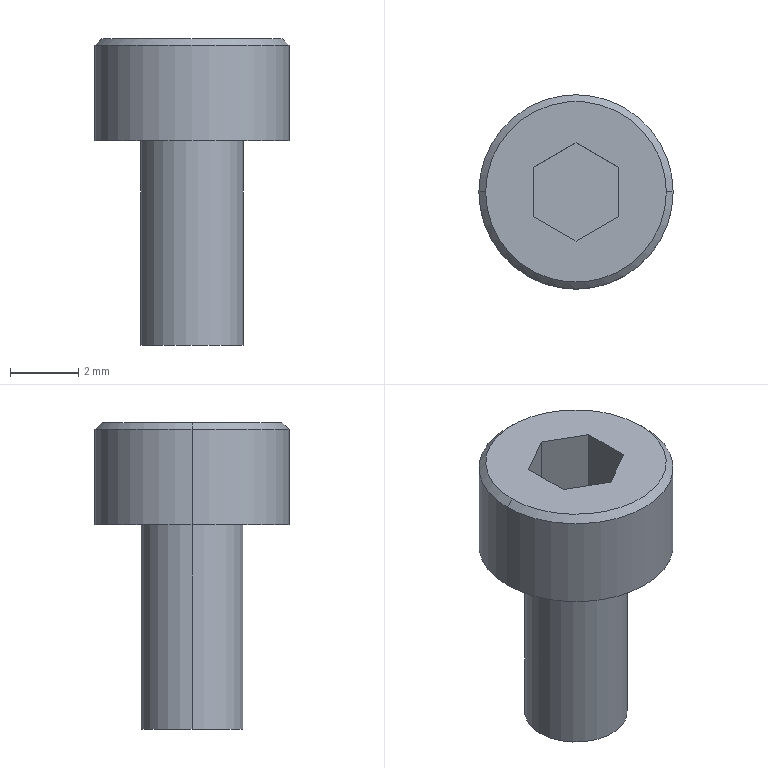Part | SolidWorks | features ICE 2, Chamfer 1, Extrusion 1 | 1 solid | 16 faces | box 5.7 x 5.7 x 9 mm | volume 102.377 mm3 | plane 10 | cylinder 4 | cone 2 | commonest cylinder face diameters 3 x2 5.7 x2
STEP:
#1=CARTESIAN_POINT('',(-1.5,0.,-6.));
#2=VERTEX_POINT('',#1);
#3=CARTESIAN_POINT('',(1.5,0.,-6.));
#4=VERTEX_POINT('',#3);
#5=CARTESIAN_POINT('',(0.,0.,-6.));
#6=DIRECTION('',(0.,0.,-1.));
#7=DIRECTION('',(-1.,0.,0.));
#8=AXIS2_PLACEMENT_3D('',#5,#6,#7);
#9=CIRCLE('',#8,1.5);
#10=EDGE_CURVE('',#2,#4,#9,.T.);
#11=ORIENTED_EDGE('',*,*,#10,.F.);
#12=CARTESIAN_POINT('',(-1.5,0.,0.));
#13=VERTEX_POINT('',#12);
#14=CARTESIAN_POINT('',(-1.5,0.,-6.));
#15=DIRECTION('',(0.,0.,1.));
#16=VECTOR('',#15,1000.);
#17=LINE('',#14,#16);
#18=EDGE_CURVE('',#2,#13,#17,.T.);
#19=ORIENTED_EDGE('',*,*,#18,.T.);
#20=CARTESIAN_POINT('',(1.5,0.,0.));
#21=VERTEX_POINT('',#20);
#22=CARTESIAN_POINT('',(0.,0.,0.));
#23=DIRECTION('',(0.,0.,-1.));
#24=DIRECTION('',(1.,0.,0.));
#25=AXIS2_PLACEMENT_3D('',#22,#23,#24);
#26=CIRCLE('',#25,1.5);
#27=EDGE_CURVE('',#13,#21,#26,.T.);
#28=ORIENTED_EDGE('',*,*,#27,.T.);
#29=CARTESIAN_POINT('',(1.5,0.,-6.));
#30=DIRECTION('',(0.,0.,1.));
#31=VECTOR('',#30,1000.);
#32=LINE('',#29,#31);
#33=EDGE_CURVE('',#4,#21,#32,.T.);
#34=ORIENTED_EDGE('',*,*,#33,.F.);
#35=EDGE_LOOP('',(#11,#19,#28,#34));
#36=FACE_OUTER_BOUND('',#35,.T.);
#37=CARTESIAN_POINT('',(0.,0.,-6.));
#38=DIRECTION('',(0.,0.,1.));
#39=DIRECTION('',(1.,0.,0.));
#40=AXIS2_PLACEMENT_3D('',#37,#38,#39);
#41=CYLINDRICAL_SURFACE('',#40,1.5);
#42=ADVANCED_FACE('',(#36),#41,.T.);
#43=CARTESIAN_POINT('',(2.65,0.,3.));
#44=VERTEX_POINT('',#43);
#45=CARTESIAN_POINT('',(-2.65,0.,3.));
#46=VERTEX_POINT('',#45);
#47=CARTESIAN_POINT('',(0.,0.,3.));
#48=DIRECTION('',(0.,0.,1.));
#49=DIRECTION('',(1.,0.,0.));
#50=AXIS2_PLACEMENT_3D('',#47,#48,#49);
#51=CIRCLE('',#50,2.65);
#52=EDGE_CURVE('',#44,#46,#51,.T.);
#53=ORIENTED_EDGE('',*,*,#52,.F.);
#54=CARTESIAN_POINT('',(2.85,0.,2.8));
#55=VERTEX_POINT('',#54);
#56=CARTESIAN_POINT('',(2.65,0.,3.));
#57=DIRECTION('',(0.7071,0.,-0.7071));
#58=VECTOR('',#57,1000.);
#59=LINE('',#56,#58);
#60=EDGE_CURVE('',#44,#55,#59,.T.);
#61=ORIENTED_EDGE('',*,*,#60,.T.);
#62=CARTESIAN_POINT('',(-2.85,0.,2.8));
#63=VERTEX_POINT('',#62);
#64=CARTESIAN_POINT('',(0.,0.,2.8));
#65=DIRECTION('',(0.,0.,-1.));
#66=DIRECTION('',(1.,0.,0.));
#67=AXIS2_PLACEMENT_3D('',#64,#65,#66);
#68=CIRCLE('',#67,2.85);
#69=EDGE_CURVE('',#63,#55,#68,.T.);
#70=ORIENTED_EDGE('',*,*,#69,.F.);
#71=CARTESIAN_POINT('',(-2.65,0.,3.));
#72=DIRECTION('',(-0.7071,0.,-0.7071));
#73=VECTOR('',#72,1000.);
#74=LINE('',#71,#73);
#75=EDGE_CURVE('',#46,#63,#74,.T.);
#76=ORIENTED_EDGE('',*,*,#75,.F.);
#77=EDGE_LOOP('',(#53,#61,#70,#76));
#78=FACE_OUTER_BOUND('',#77,.T.);
#79=CARTESIAN_POINT('',(0.,0.,3.));
#80=DIRECTION('',(0.,0.,-1.));
#81=DIRECTION('',(-1.,0.,0.));
#82=AXIS2_PLACEMENT_3D('',#79,#80,#81);
#83=CONICAL_SURFACE('',#82,2.65,0.7854);
#84=ADVANCED_FACE('',(#78),#83,.T.);
#85=ORIENTED_EDGE('',*,*,#69,.T.);
#86=CARTESIAN_POINT('',(2.85,0.,0.));
#87=VERTEX_POINT('',#86);
#88=CARTESIAN_POINT('',(2.85,0.,3.));
#89=DIRECTION('',(0.,0.,-1.));
#90=VECTOR('',#89,1000.);
#91=LINE('',#88,#90);
#92=EDGE_CURVE('',#55,#87,#91,.T.);
#93=ORIENTED_EDGE('',*,*,#92,.T.);
#94=CARTESIAN_POINT('',(-2.85,0.,0.));
#95=VERTEX_POINT('',#94);
#96=CARTESIAN_POINT('',(0.,0.,0.));
#97=DIRECTION('',(0.,0.,1.));
#98=DIRECTION('',(1.,0.,0.));
#99=AXIS2_PLACEMENT_3D('',#96,#97,#98);
#100=CIRCLE('',#99,2.85);
#101=EDGE_CURVE('',#87,#95,#100,.T.);
#102=ORIENTED_EDGE('',*,*,#101,.T.);
#103=CARTESIAN_POINT('',(-2.85,0.,3.));
#104=DIRECTION('',(0.,0.,-1.));
#105=VECTOR('',#104,1000.);
#106=LINE('',#103,#105);
#107=EDGE_CURVE('',#63,#95,#106,.T.);
#108=ORIENTED_EDGE('',*,*,#107,.F.);
#109=EDGE_LOOP('',(#85,#93,#102,#108));
#110=FACE_OUTER_BOUND('',#109,.T.);
#111=CARTESIAN_POINT('',(0.,0.,3.));
#112=DIRECTION('',(0.,0.,-1.));
#113=DIRECTION('',(-1.,0.,0.));
#114=AXIS2_PLACEMENT_3D('',#111,#112,#113);
#115=CYLINDRICAL_SURFACE('',#114,2.85);
#116=ADVANCED_FACE('',(#110),#115,.T.);
#117=CARTESIAN_POINT('',(0.,0.,0.));
#118=DIRECTION('',(0.,0.,1.));
#119=DIRECTION('',(1.,0.,0.));
#120=AXIS2_PLACEMENT_3D('',#117,#118,#119);
#121=CIRCLE('',#120,2.85);
#122=EDGE_CURVE('',#95,#87,#121,.T.);
#123=ORIENTED_EDGE('',*,*,#122,.F.);
#124=ORIENTED_EDGE('',*,*,#101,.F.);
#125=EDGE_LOOP('',(#123,#124));
#126=FACE_OUTER_BOUND('',#125,.T.);
#127=CARTESIAN_POINT('',(0.,0.,0.));
#128=DIRECTION('',(0.,0.,-1.));
#129=DIRECTION('',(1.,0.,0.));
#130=AXIS2_PLACEMENT_3D('',#127,#128,#129);
#131=CIRCLE('',#130,1.5);
#132=EDGE_CURVE('',#21,#13,#131,.T.);
#133=ORIENTED_EDGE('',*,*,#132,.F.);
#134=ORIENTED_EDGE('',*,*,#27,.F.);
#135=EDGE_LOOP('',(#133,#134));
#136=FACE_BOUND('',#135,.T.);
#137=CARTESIAN_POINT('',(0.,0.,0.));
#138=DIRECTION('',(0.,0.,1.));
#139=DIRECTION('',(1.,0.,0.));
#140=AXIS2_PLACEMENT_3D('',#137,#138,#139);
#141=PLANE('',#140);
#142=ADVANCED_FACE('',(#126,#136),#141,.F.);
#143=ORIENTED_EDGE('',*,*,#92,.F.);
#144=CARTESIAN_POINT('',(0.,0.,2.8));
#145=DIRECTION('',(0.,0.,-1.));
#146=DIRECTION('',(1.,0.,0.));
#147=AXIS2_PLACEMENT_3D('',#144,#145,#146);
#148=CIRCLE('',#147,2.85);
#149=EDGE_CURVE('',#55,#63,#148,.T.);
#150=ORIENTED_EDGE('',*,*,#149,.T.);
#151=ORIENTED_EDGE('',*,*,#107,.T.);
#152=ORIENTED_EDGE('',*,*,#122,.T.);
#153=EDGE_LOOP('',(#143,#150,#151,#152));
#154=FACE_OUTER_BOUND('',#153,.T.);
#155=CARTESIAN_POINT('',(0.,0.,3.));
#156=DIRECTION('',(0.,0.,-1.));
#157=DIRECTION('',(-1.,0.,0.));
#158=AXIS2_PLACEMENT_3D('',#155,#156,#157);
#159=CYLINDRICAL_SURFACE('',#158,2.85);
#160=ADVANCED_FACE('',(#154),#159,.T.);
#161=CARTESIAN_POINT('',(0.,0.,3.));
#162=DIRECTION('',(0.,0.,1.));
#163=DIRECTION('',(1.,0.,0.));
#164=AXIS2_PLACEMENT_3D('',#161,#162,#163);
#165=CIRCLE('',#164,2.65);
#166=EDGE_CURVE('',#46,#44,#165,.T.);
#167=ORIENTED_EDGE('',*,*,#166,.T.);
#168=ORIENTED_EDGE('',*,*,#52,.T.);
#169=EDGE_LOOP('',(#167,#168));
#170=FACE_OUTER_BOUND('',#169,.T.);
#171=CARTESIAN_POINT('',(1.25,0.7217,3.));
#172=VERTEX_POINT('',#171);
#173=CARTESIAN_POINT('',(0.,1.443,3.));
#174=VERTEX_POINT('',#173);
#175=CARTESIAN_POINT('',(1.25,0.7217,3.));
#176=DIRECTION('',(-0.866,0.5,0.));
#177=VECTOR('',#176,1000.);
#178=LINE('',#175,#177);
#179=EDGE_CURVE('',#172,#174,#178,.T.);
#180=ORIENTED_EDGE('',*,*,#179,.F.);
#181=CARTESIAN_POINT('',(1.25,-0.7217,3.));
#182=VERTEX_POINT('',#181);
#183=CARTESIAN_POINT('',(1.25,-0.7217,3.));
#184=DIRECTION('',(0.,1.,0.));
#185=VECTOR('',#184,1000.);
#186=LINE('',#183,#185);
#187=EDGE_CURVE('',#182,#172,#186,.T.);
#188=ORIENTED_EDGE('',*,*,#187,.F.);
#189=CARTESIAN_POINT('',(0.,-1.443,3.));
#190=VERTEX_POINT('',#189);
#191=CARTESIAN_POINT('',(0.,-1.443,3.));
#192=DIRECTION('',(0.866,0.5,0.));
#193=VECTOR('',#192,1000.);
#194=LINE('',#191,#193);
#195=EDGE_CURVE('',#190,#182,#194,.T.);
#196=ORIENTED_EDGE('',*,*,#195,.F.);
#197=CARTESIAN_POINT('',(-1.25,-0.7217,3.));
#198=VERTEX_POINT('',#197);
#199=CARTESIAN_POINT('',(-1.25,-0.7217,3.));
#200=DIRECTION('',(0.866,-0.5,0.));
#201=VECTOR('',#200,1000.);
#202=LINE('',#199,#201);
#203=EDGE_CURVE('',#198,#190,#202,.T.);
#204=ORIENTED_EDGE('',*,*,#203,.F.);
#205=CARTESIAN_POINT('',(-1.25,0.7217,3.));
#206=VERTEX_POINT('',#205);
#207=CARTESIAN_POINT('',(-1.25,0.7217,3.));
#208=DIRECTION('',(0.,-1.,0.));
#209=VECTOR('',#208,1000.);
#210=LINE('',#207,#209);
#211=EDGE_CURVE('',#206,#198,#210,.T.);
#212=ORIENTED_EDGE('',*,*,#211,.F.);
#213=CARTESIAN_POINT('',(0.,1.443,3.));
#214=DIRECTION('',(-0.866,-0.5,0.));
#215=VECTOR('',#214,1000.);
#216=LINE('',#213,#215);
#217=EDGE_CURVE('',#174,#206,#216,.T.);
#218=ORIENTED_EDGE('',*,*,#217,.F.);
#219=EDGE_LOOP('',(#180,#188,#196,#204,#212,#218));
#220=FACE_BOUND('',#219,.T.);
#221=CARTESIAN_POINT('',(0.,0.,3.));
#222=DIRECTION('',(0.,0.,1.));
#223=DIRECTION('',(1.,0.,0.));
#224=AXIS2_PLACEMENT_3D('',#221,#222,#223);
#225=PLANE('',#224);
#226=ADVANCED_FACE('',(#170,#220),#225,.T.);
#227=CARTESIAN_POINT('',(1.25,0.7217,0.));
#228=VERTEX_POINT('',#227);
#229=CARTESIAN_POINT('',(1.25,0.7217,-1.));
#230=DIRECTION('',(0.,0.,1.));
#231=VECTOR('',#230,1000.);
#232=LINE('',#229,#231);
#233=EDGE_CURVE('',#228,#172,#232,.T.);
#234=ORIENTED_EDGE('',*,*,#233,.T.);
#235=ORIENTED_EDGE('',*,*,#179,.T.);
#236=CARTESIAN_POINT('',(0.,1.443,0.));
#237=VERTEX_POINT('',#236);
#238=CARTESIAN_POINT('',(0.,1.443,-1.));
#239=DIRECTION('',(0.,0.,1.));
#240=VECTOR('',#239,1000.);
#241=LINE('',#238,#240);
#242=EDGE_CURVE('',#237,#174,#241,.T.);
#243=ORIENTED_EDGE('',*,*,#242,.F.);
#244=CARTESIAN_POINT('',(0.625,1.083,0.));
#245=DIRECTION('',(-0.866,0.5,0.));
#246=VECTOR('',#245,1000.);
#247=LINE('',#244,#246);
#248=EDGE_CURVE('',#228,#237,#247,.T.);
#249=ORIENTED_EDGE('',*,*,#248,.F.);
#250=EDGE_LOOP('',(#234,#235,#243,#249));
#251=FACE_OUTER_BOUND('',#250,.T.);
#252=CARTESIAN_POINT('',(1.25,0.7217,-1.));
#253=DIRECTION('',(0.5,0.866,0.));
#254=DIRECTION('',(-0.866,0.5,0.));
#255=AXIS2_PLACEMENT_3D('',#252,#253,#254);
#256=PLANE('',#255);
#257=ADVANCED_FACE('',(#251),#256,.F.);
#258=CARTESIAN_POINT('',(1.25,-0.7217,0.));
#259=VERTEX_POINT('',#258);
#260=CARTESIAN_POINT('',(1.25,-0.7217,-1.));
#261=DIRECTION('',(0.,0.,1.));
#262=VECTOR('',#261,1000.);
#263=LINE('',#260,#262);
#264=EDGE_CURVE('',#259,#182,#263,.T.);
#265=ORIENTED_EDGE('',*,*,#264,.T.);
#266=ORIENTED_EDGE('',*,*,#187,.T.);
#267=ORIENTED_EDGE('',*,*,#233,.F.);
#268=CARTESIAN_POINT('',(1.25,0.,0.));
#269=DIRECTION('',(0.,1.,0.));
#270=VECTOR('',#269,1000.);
#271=LINE('',#268,#270);
#272=EDGE_CURVE('',#259,#228,#271,.T.);
#273=ORIENTED_EDGE('',*,*,#272,.F.);
#274=EDGE_LOOP('',(#265,#266,#267,#273));
#275=FACE_OUTER_BOUND('',#274,.T.);
#276=CARTESIAN_POINT('',(1.25,-0.7217,-1.));
#277=DIRECTION('',(1.,0.,0.));
#278=DIRECTION('',(0.,1.,0.));
#279=AXIS2_PLACEMENT_3D('',#276,#277,#278);
#280=PLANE('',#279);
#281=ADVANCED_FACE('',(#275),#280,.F.);
#282=CARTESIAN_POINT('',(0.,-1.443,0.));
#283=VERTEX_POINT('',#282);
#284=CARTESIAN_POINT('',(0.,-1.443,-1.));
#285=DIRECTION('',(0.,0.,1.));
#286=VECTOR('',#285,1000.);
#287=LINE('',#284,#286);
#288=EDGE_CURVE('',#283,#190,#287,.T.);
#289=ORIENTED_EDGE('',*,*,#288,.T.);
#290=ORIENTED_EDGE('',*,*,#195,.T.);
#291=ORIENTED_EDGE('',*,*,#264,.F.);
#292=CARTESIAN_POINT('',(0.625,-1.083,0.));
#293=DIRECTION('',(0.866,0.5,0.));
#294=VECTOR('',#293,1000.);
#295=LINE('',#292,#294);
#296=EDGE_CURVE('',#283,#259,#295,.T.);
#297=ORIENTED_EDGE('',*,*,#296,.F.);
#298=EDGE_LOOP('',(#289,#290,#291,#297));
#299=FACE_OUTER_BOUND('',#298,.T.);
#300=CARTESIAN_POINT('',(0.,-1.443,-1.));
#301=DIRECTION('',(0.5,-0.866,0.));
#302=DIRECTION('',(0.866,0.5,0.));
#303=AXIS2_PLACEMENT_3D('',#300,#301,#302);
#304=PLANE('',#303);
#305=ADVANCED_FACE('',(#299),#304,.F.);
#306=CARTESIAN_POINT('',(-1.25,-0.7217,0.));
#307=VERTEX_POINT('',#306);
#308=CARTESIAN_POINT('',(-1.25,-0.7217,-1.));
#309=DIRECTION('',(0.,0.,1.));
#310=VECTOR('',#309,1000.);
#311=LINE('',#308,#310);
#312=EDGE_CURVE('',#307,#198,#311,.T.);
#313=ORIENTED_EDGE('',*,*,#312,.T.);
#314=ORIENTED_EDGE('',*,*,#203,.T.);
#315=ORIENTED_EDGE('',*,*,#288,.F.);
#316=CARTESIAN_POINT('',(-0.625,-1.083,0.));
#317=DIRECTION('',(0.866,-0.5,0.));
#318=VECTOR('',#317,1000.);
#319=LINE('',#316,#318);
#320=EDGE_CURVE('',#307,#283,#319,.T.);
#321=ORIENTED_EDGE('',*,*,#320,.F.);
#322=EDGE_LOOP('',(#313,#314,#315,#321));
#323=FACE_OUTER_BOUND('',#322,.T.);
#324=CARTESIAN_POINT('',(-1.25,-0.7217,-1.));
#325=DIRECTION('',(-0.5,-0.866,0.));
#326=DIRECTION('',(0.866,-0.5,0.));
#327=AXIS2_PLACEMENT_3D('',#324,#325,#326);
#328=PLANE('',#327);
#329=ADVANCED_FACE('',(#323),#328,.F.);
#330=CARTESIAN_POINT('',(-1.25,0.7217,0.));
#331=VERTEX_POINT('',#330);
#332=CARTESIAN_POINT('',(-1.25,0.7217,-1.));
#333=DIRECTION('',(0.,0.,1.));
#334=VECTOR('',#333,1000.);
#335=LINE('',#332,#334);
#336=EDGE_CURVE('',#331,#206,#335,.T.);
#337=ORIENTED_EDGE('',*,*,#336,.T.);
#338=ORIENTED_EDGE('',*,*,#211,.T.);
#339=ORIENTED_EDGE('',*,*,#312,.F.);
#340=CARTESIAN_POINT('',(-1.25,0.,0.));
#341=DIRECTION('',(0.,-1.,0.));
#342=VECTOR('',#341,1000.);
#343=LINE('',#340,#342);
#344=EDGE_CURVE('',#331,#307,#343,.T.);
#345=ORIENTED_EDGE('',*,*,#344,.F.);
#346=EDGE_LOOP('',(#337,#338,#339,#345));
#347=FACE_OUTER_BOUND('',#346,.T.);
#348=CARTESIAN_POINT('',(-1.25,0.7217,-1.));
#349=DIRECTION('',(-1.,0.,0.));
#350=DIRECTION('',(0.,0.,1.));
#351=AXIS2_PLACEMENT_3D('',#348,#349,#350);
#352=PLANE('',#351);
#353=ADVANCED_FACE('',(#347),#352,.F.);
#354=ORIENTED_EDGE('',*,*,#242,.T.);
#355=ORIENTED_EDGE('',*,*,#217,.T.);
#356=ORIENTED_EDGE('',*,*,#336,.F.);
#357=CARTESIAN_POINT('',(-0.625,1.083,0.));
#358=DIRECTION('',(-0.866,-0.5,0.));
#359=VECTOR('',#358,1000.);
#360=LINE('',#357,#359);
#361=EDGE_CURVE('',#237,#331,#360,.T.);
#362=ORIENTED_EDGE('',*,*,#361,.F.);
#363=EDGE_LOOP('',(#354,#355,#356,#362));
#364=FACE_OUTER_BOUND('',#363,.T.);
#365=CARTESIAN_POINT('',(0.,1.443,-1.));
#366=DIRECTION('',(-0.5,0.866,0.));
#367=DIRECTION('',(-0.866,-0.5,0.));
#368=AXIS2_PLACEMENT_3D('',#365,#366,#367);
#369=PLANE('',#368);
#370=ADVANCED_FACE('',(#364),#369,.F.);
#371=ORIENTED_EDGE('',*,*,#60,.F.);
#372=ORIENTED_EDGE('',*,*,#166,.F.);
#373=ORIENTED_EDGE('',*,*,#75,.T.);
#374=ORIENTED_EDGE('',*,*,#149,.F.);
#375=EDGE_LOOP('',(#371,#372,#373,#374));
#376=FACE_OUTER_BOUND('',#375,.T.);
#377=CARTESIAN_POINT('',(0.,0.,3.));
#378=DIRECTION('',(0.,0.,-1.));
#379=DIRECTION('',(-1.,0.,0.));
#380=AXIS2_PLACEMENT_3D('',#377,#378,#379);
#381=CONICAL_SURFACE('',#380,2.65,0.7854);
#382=ADVANCED_FACE('',(#376),#381,.T.);
#383=ORIENTED_EDGE('',*,*,#272,.T.);
#384=ORIENTED_EDGE('',*,*,#248,.T.);
#385=ORIENTED_EDGE('',*,*,#361,.T.);
#386=ORIENTED_EDGE('',*,*,#344,.T.);
#387=ORIENTED_EDGE('',*,*,#320,.T.);
#388=ORIENTED_EDGE('',*,*,#296,.T.);
#389=EDGE_LOOP('',(#383,#384,#385,#386,#387,#388));
#390=FACE_OUTER_BOUND('',#389,.T.);
#391=CARTESIAN_POINT('',(0.,0.,0.));
#392=DIRECTION('',(0.,0.,-1.));
#393=DIRECTION('',(-1.,0.,0.));
#394=AXIS2_PLACEMENT_3D('',#391,#392,#393);
#395=PLANE('',#394);
#396=ADVANCED_FACE('',(#390),#395,.F.);
#397=ORIENTED_EDGE('',*,*,#18,.F.);
#398=CARTESIAN_POINT('',(0.,0.,-6.));
#399=DIRECTION('',(0.,0.,-1.));
#400=DIRECTION('',(-1.,0.,0.));
#401=AXIS2_PLACEMENT_3D('',#398,#399,#400);
#402=CIRCLE('',#401,1.5);
#403=EDGE_CURVE('',#4,#2,#402,.T.);
#404=ORIENTED_EDGE('',*,*,#403,.F.);
#405=ORIENTED_EDGE('',*,*,#33,.T.);
#406=ORIENTED_EDGE('',*,*,#132,.T.);
#407=EDGE_LOOP('',(#397,#404,#405,#406));
#408=FACE_OUTER_BOUND('',#407,.T.);
#409=CARTESIAN_POINT('',(0.,0.,-6.));
#410=DIRECTION('',(0.,0.,1.));
#411=DIRECTION('',(1.,0.,0.));
#412=AXIS2_PLACEMENT_3D('',#409,#410,#411);
#413=CYLINDRICAL_SURFACE('',#412,1.5);
#414=ADVANCED_FACE('',(#408),#413,.T.);
#415=ORIENTED_EDGE('',*,*,#403,.T.);
#416=ORIENTED_EDGE('',*,*,#10,.T.);
#417=EDGE_LOOP('',(#415,#416));
#418=FACE_OUTER_BOUND('',#417,.T.);
#419=CARTESIAN_POINT('',(0.,0.,-6.));
#420=DIRECTION('',(0.,0.,-1.));
#421=DIRECTION('',(-1.,0.,0.));
#422=AXIS2_PLACEMENT_3D('',#419,#420,#421);
#423=PLANE('',#422);
#424=ADVANCED_FACE('',(#418),#423,.T.);
#425=CLOSED_SHELL('',(#42,#84,#116,#142,#160,#226,#257,#281,#305,#329,#353,#370,#382,#396,#414,#424));
#426=MANIFOLD_SOLID_BREP('',#425);
#427=CARTESIAN_POINT('',(0.,0.,0.));
#428=DIRECTION('',(0.,0.,1.));
#429=DIRECTION('',(1.,0.,0.));
#430=AXIS2_PLACEMENT_3D('',#427,#428,#429);
#431=(LENGTH_UNIT()NAMED_UNIT(*)SI_UNIT(.MILLI.,.METRE.));
#432=UNCERTAINTY_MEASURE_WITH_UNIT(LENGTH_MEASURE(0.00001),#431,'','');
#433=(NAMED_UNIT(*)PLANE_ANGLE_UNIT()SI_UNIT($,.RADIAN.));
#434=(NAMED_UNIT(*)SI_UNIT($,.STERADIAN.)SOLID_ANGLE_UNIT());
#435=(GEOMETRIC_REPRESENTATION_CONTEXT(3)GLOBAL_UNCERTAINTY_ASSIGNED_CONTEXT((#432))GLOBAL_UNIT_ASSIGNED_CONTEXT((#431,#433,#434))REPRESENTATION_CONTEXT('',''));
#436=ADVANCED_BREP_SHAPE_REPRESENTATION('',(#426,#430),#435);